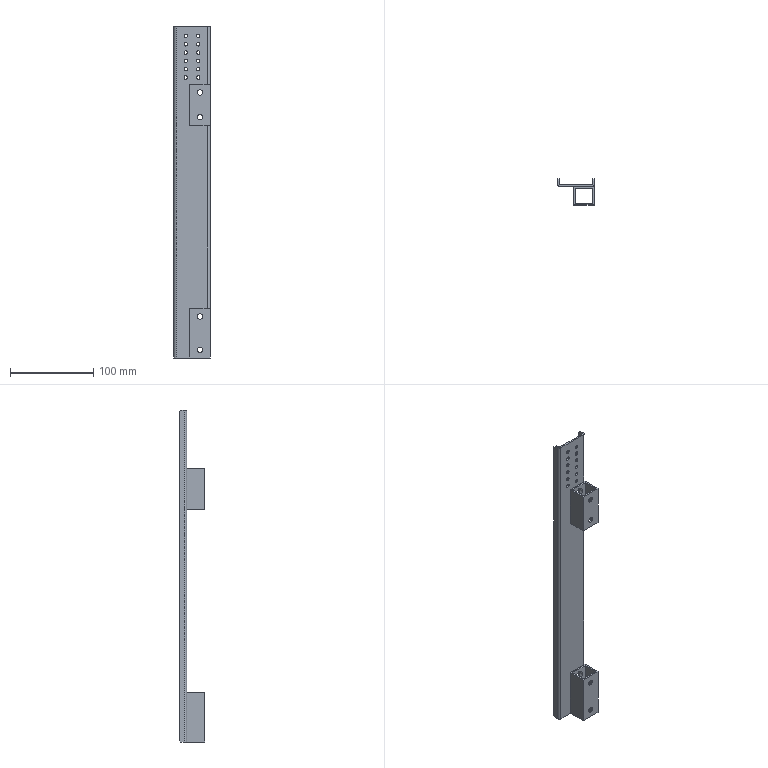Part | STEP file | 11-FG-B08911 | 1 solid | 85 faces | box 44 x 31 x 400 mm | volume 61704 mm3 | cylinder 44 | plane 41 | commonest cylinder face diameters 4.2 x24 6.5 x8 12 x8 1.473 x2 5.473 x2